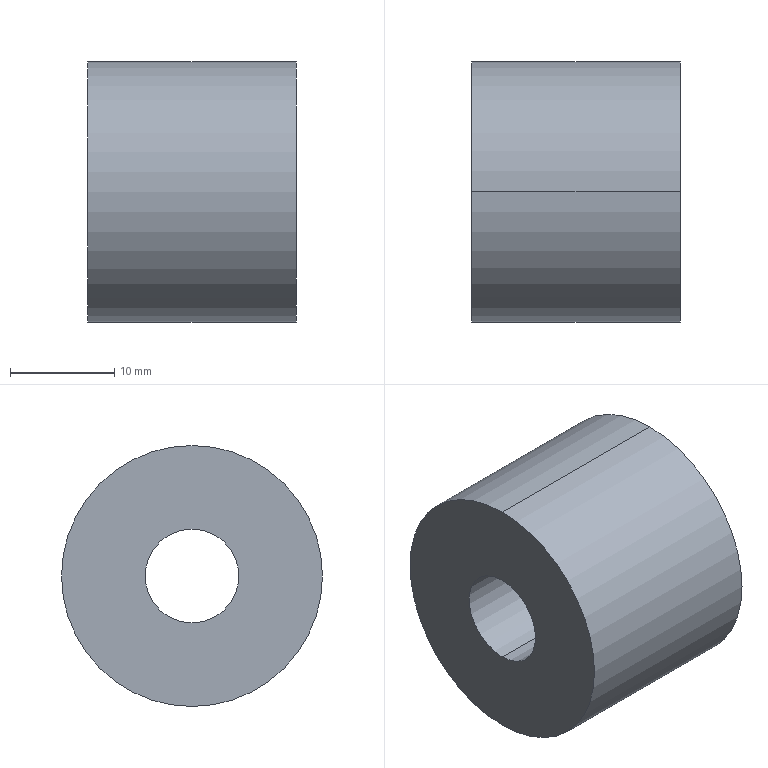Part | SolidWorks | features Extrusion 1, HoleWzd 1 | 1 solid | 9 faces | box 20 x 25 x 25 mm | volume 7188 mm3 | cylinder 6 | plane 3 | commonest cylinder face diameters 9 x2 15 x2 25 x2
STEP:
#1=CARTESIAN_POINT('',(8.,0.,7.5));
#2=VERTEX_POINT('',#1);
#3=CARTESIAN_POINT('',(8.,0.,-7.5));
#4=VERTEX_POINT('',#3);
#5=CARTESIAN_POINT('',(8.,0.,0.));
#6=DIRECTION('',(1.,0.,0.));
#7=DIRECTION('',(0.,0.,-1.));
#8=AXIS2_PLACEMENT_3D('',#5,#6,#7);
#9=CIRCLE('',#8,7.5);
#10=EDGE_CURVE('',#2,#4,#9,.T.);
#11=ORIENTED_EDGE('',*,*,#10,.F.);
#12=CARTESIAN_POINT('',(20.,0.,7.5));
#13=VERTEX_POINT('',#12);
#14=CARTESIAN_POINT('',(20.,0.,7.5));
#15=DIRECTION('',(1.,0.,0.));
#16=VECTOR('',#15,1000.);
#17=LINE('',#14,#16);
#18=EDGE_CURVE('',#2,#13,#17,.T.);
#19=ORIENTED_EDGE('',*,*,#18,.T.);
#20=CARTESIAN_POINT('',(20.,0.,-7.5));
#21=VERTEX_POINT('',#20);
#22=CARTESIAN_POINT('',(20.,0.,0.));
#23=DIRECTION('',(1.,0.,0.));
#24=DIRECTION('',(0.,0.,-1.));
#25=AXIS2_PLACEMENT_3D('',#22,#23,#24);
#26=CIRCLE('',#25,7.5);
#27=EDGE_CURVE('',#13,#21,#26,.T.);
#28=ORIENTED_EDGE('',*,*,#27,.T.);
#29=CARTESIAN_POINT('',(20.,0.,-7.5));
#30=DIRECTION('',(1.,0.,0.));
#31=VECTOR('',#30,1000.);
#32=LINE('',#29,#31);
#33=EDGE_CURVE('',#4,#21,#32,.T.);
#34=ORIENTED_EDGE('',*,*,#33,.F.);
#35=EDGE_LOOP('',(#11,#19,#28,#34));
#36=FACE_OUTER_BOUND('',#35,.T.);
#37=CARTESIAN_POINT('',(20.,0.,0.));
#38=DIRECTION('',(1.,0.,0.));
#39=DIRECTION('',(0.,0.,-1.));
#40=AXIS2_PLACEMENT_3D('',#37,#38,#39);
#41=CYLINDRICAL_SURFACE('',#40,7.5);
#42=ADVANCED_FACE('',(#36),#41,.F.);
#43=CARTESIAN_POINT('',(0.,0.,4.5));
#44=VERTEX_POINT('',#43);
#45=CARTESIAN_POINT('',(0.,0.,-4.5));
#46=VERTEX_POINT('',#45);
#47=CARTESIAN_POINT('',(0.,0.,0.));
#48=DIRECTION('',(1.,0.,0.));
#49=DIRECTION('',(0.,0.,-1.));
#50=AXIS2_PLACEMENT_3D('',#47,#48,#49);
#51=CIRCLE('',#50,4.5);
#52=EDGE_CURVE('',#44,#46,#51,.T.);
#53=ORIENTED_EDGE('',*,*,#52,.F.);
#54=CARTESIAN_POINT('',(8.,0.,4.5));
#55=VERTEX_POINT('',#54);
#56=CARTESIAN_POINT('',(20.,0.,4.5));
#57=DIRECTION('',(1.,0.,0.));
#58=VECTOR('',#57,1000.);
#59=LINE('',#56,#58);
#60=EDGE_CURVE('',#44,#55,#59,.T.);
#61=ORIENTED_EDGE('',*,*,#60,.T.);
#62=CARTESIAN_POINT('',(8.,0.,-4.5));
#63=VERTEX_POINT('',#62);
#64=CARTESIAN_POINT('',(8.,0.,0.));
#65=DIRECTION('',(1.,0.,0.));
#66=DIRECTION('',(0.,0.,-1.));
#67=AXIS2_PLACEMENT_3D('',#64,#65,#66);
#68=CIRCLE('',#67,4.5);
#69=EDGE_CURVE('',#55,#63,#68,.T.);
#70=ORIENTED_EDGE('',*,*,#69,.T.);
#71=CARTESIAN_POINT('',(20.,0.,-4.5));
#72=DIRECTION('',(1.,0.,0.));
#73=VECTOR('',#72,1000.);
#74=LINE('',#71,#73);
#75=EDGE_CURVE('',#46,#63,#74,.T.);
#76=ORIENTED_EDGE('',*,*,#75,.F.);
#77=EDGE_LOOP('',(#53,#61,#70,#76));
#78=FACE_OUTER_BOUND('',#77,.T.);
#79=CARTESIAN_POINT('',(20.,0.,0.));
#80=DIRECTION('',(1.,0.,0.));
#81=DIRECTION('',(0.,0.,-1.));
#82=AXIS2_PLACEMENT_3D('',#79,#80,#81);
#83=CYLINDRICAL_SURFACE('',#82,4.5);
#84=ADVANCED_FACE('',(#78),#83,.F.);
#85=CARTESIAN_POINT('',(20.,0.,-12.5));
#86=VERTEX_POINT('',#85);
#87=CARTESIAN_POINT('',(20.,0.,12.5));
#88=VERTEX_POINT('',#87);
#89=CARTESIAN_POINT('',(20.,0.,0.));
#90=DIRECTION('',(1.,0.,0.));
#91=DIRECTION('',(0.,0.,-1.));
#92=AXIS2_PLACEMENT_3D('',#89,#90,#91);
#93=CIRCLE('',#92,12.5);
#94=EDGE_CURVE('',#86,#88,#93,.T.);
#95=ORIENTED_EDGE('',*,*,#94,.F.);
#96=CARTESIAN_POINT('',(0.,0.,-12.5));
#97=VERTEX_POINT('',#96);
#98=CARTESIAN_POINT('',(20.,0.,-12.5));
#99=DIRECTION('',(-1.,0.,0.));
#100=VECTOR('',#99,1000.);
#101=LINE('',#98,#100);
#102=EDGE_CURVE('',#86,#97,#101,.T.);
#103=ORIENTED_EDGE('',*,*,#102,.T.);
#104=CARTESIAN_POINT('',(0.,0.,12.5));
#105=VERTEX_POINT('',#104);
#106=CARTESIAN_POINT('',(0.,0.,0.));
#107=DIRECTION('',(1.,0.,0.));
#108=DIRECTION('',(0.,0.,-1.));
#109=AXIS2_PLACEMENT_3D('',#106,#107,#108);
#110=CIRCLE('',#109,12.5);
#111=EDGE_CURVE('',#97,#105,#110,.T.);
#112=ORIENTED_EDGE('',*,*,#111,.T.);
#113=CARTESIAN_POINT('',(20.,0.,12.5));
#114=DIRECTION('',(-1.,0.,0.));
#115=VECTOR('',#114,1000.);
#116=LINE('',#113,#115);
#117=EDGE_CURVE('',#88,#105,#116,.T.);
#118=ORIENTED_EDGE('',*,*,#117,.F.);
#119=EDGE_LOOP('',(#95,#103,#112,#118));
#120=FACE_OUTER_BOUND('',#119,.T.);
#121=CARTESIAN_POINT('',(20.,0.,0.));
#122=DIRECTION('',(-1.,0.,0.));
#123=DIRECTION('',(0.,0.,1.));
#124=AXIS2_PLACEMENT_3D('',#121,#122,#123);
#125=CYLINDRICAL_SURFACE('',#124,12.5);
#126=ADVANCED_FACE('',(#120),#125,.T.);
#127=ORIENTED_EDGE('',*,*,#102,.F.);
#128=CARTESIAN_POINT('',(20.,0.,0.));
#129=DIRECTION('',(1.,0.,0.));
#130=DIRECTION('',(0.,0.,-1.));
#131=AXIS2_PLACEMENT_3D('',#128,#129,#130);
#132=CIRCLE('',#131,12.5);
#133=EDGE_CURVE('',#88,#86,#132,.T.);
#134=ORIENTED_EDGE('',*,*,#133,.F.);
#135=ORIENTED_EDGE('',*,*,#117,.T.);
#136=CARTESIAN_POINT('',(0.,0.,0.));
#137=DIRECTION('',(1.,0.,0.));
#138=DIRECTION('',(0.,0.,-1.));
#139=AXIS2_PLACEMENT_3D('',#136,#137,#138);
#140=CIRCLE('',#139,12.5);
#141=EDGE_CURVE('',#105,#97,#140,.T.);
#142=ORIENTED_EDGE('',*,*,#141,.T.);
#143=EDGE_LOOP('',(#127,#134,#135,#142));
#144=FACE_OUTER_BOUND('',#143,.T.);
#145=CARTESIAN_POINT('',(20.,0.,0.));
#146=DIRECTION('',(-1.,0.,0.));
#147=DIRECTION('',(0.,0.,1.));
#148=AXIS2_PLACEMENT_3D('',#145,#146,#147);
#149=CYLINDRICAL_SURFACE('',#148,12.5);
#150=ADVANCED_FACE('',(#144),#149,.T.);
#151=CARTESIAN_POINT('',(20.,0.,0.));
#152=DIRECTION('',(1.,0.,0.));
#153=DIRECTION('',(0.,0.,-1.));
#154=AXIS2_PLACEMENT_3D('',#151,#152,#153);
#155=CIRCLE('',#154,7.5);
#156=EDGE_CURVE('',#21,#13,#155,.T.);
#157=ORIENTED_EDGE('',*,*,#156,.F.);
#158=ORIENTED_EDGE('',*,*,#27,.F.);
#159=EDGE_LOOP('',(#157,#158));
#160=FACE_BOUND('',#159,.T.);
#161=ORIENTED_EDGE('',*,*,#133,.T.);
#162=ORIENTED_EDGE('',*,*,#94,.T.);
#163=EDGE_LOOP('',(#161,#162));
#164=FACE_OUTER_BOUND('',#163,.T.);
#165=CARTESIAN_POINT('',(20.,0.,0.));
#166=DIRECTION('',(1.,0.,0.));
#167=DIRECTION('',(0.,0.,-1.));
#168=AXIS2_PLACEMENT_3D('',#165,#166,#167);
#169=PLANE('',#168);
#170=ADVANCED_FACE('',(#160,#164),#169,.T.);
#171=CARTESIAN_POINT('',(0.,0.,0.));
#172=DIRECTION('',(1.,0.,0.));
#173=DIRECTION('',(0.,0.,-1.));
#174=AXIS2_PLACEMENT_3D('',#171,#172,#173);
#175=CIRCLE('',#174,4.5);
#176=EDGE_CURVE('',#46,#44,#175,.T.);
#177=ORIENTED_EDGE('',*,*,#176,.T.);
#178=ORIENTED_EDGE('',*,*,#52,.T.);
#179=EDGE_LOOP('',(#177,#178));
#180=FACE_BOUND('',#179,.T.);
#181=ORIENTED_EDGE('',*,*,#141,.F.);
#182=ORIENTED_EDGE('',*,*,#111,.F.);
#183=EDGE_LOOP('',(#181,#182));
#184=FACE_OUTER_BOUND('',#183,.T.);
#185=CARTESIAN_POINT('',(0.,0.,0.));
#186=DIRECTION('',(1.,0.,0.));
#187=DIRECTION('',(0.,0.,-1.));
#188=AXIS2_PLACEMENT_3D('',#185,#186,#187);
#189=PLANE('',#188);
#190=ADVANCED_FACE('',(#180,#184),#189,.F.);
#191=ORIENTED_EDGE('',*,*,#60,.F.);
#192=ORIENTED_EDGE('',*,*,#176,.F.);
#193=ORIENTED_EDGE('',*,*,#75,.T.);
#194=CARTESIAN_POINT('',(8.,0.,0.));
#195=DIRECTION('',(1.,0.,0.));
#196=DIRECTION('',(0.,0.,-1.));
#197=AXIS2_PLACEMENT_3D('',#194,#195,#196);
#198=CIRCLE('',#197,4.5);
#199=EDGE_CURVE('',#63,#55,#198,.T.);
#200=ORIENTED_EDGE('',*,*,#199,.T.);
#201=EDGE_LOOP('',(#191,#192,#193,#200));
#202=FACE_OUTER_BOUND('',#201,.T.);
#203=CARTESIAN_POINT('',(20.,0.,0.));
#204=DIRECTION('',(1.,0.,0.));
#205=DIRECTION('',(0.,0.,-1.));
#206=AXIS2_PLACEMENT_3D('',#203,#204,#205);
#207=CYLINDRICAL_SURFACE('',#206,4.5);
#208=ADVANCED_FACE('',(#202),#207,.F.);
#209=ORIENTED_EDGE('',*,*,#199,.F.);
#210=ORIENTED_EDGE('',*,*,#69,.F.);
#211=EDGE_LOOP('',(#209,#210));
#212=FACE_BOUND('',#211,.T.);
#213=CARTESIAN_POINT('',(8.,0.,0.));
#214=DIRECTION('',(1.,0.,0.));
#215=DIRECTION('',(0.,0.,-1.));
#216=AXIS2_PLACEMENT_3D('',#213,#214,#215);
#217=CIRCLE('',#216,7.5);
#218=EDGE_CURVE('',#4,#2,#217,.T.);
#219=ORIENTED_EDGE('',*,*,#218,.T.);
#220=ORIENTED_EDGE('',*,*,#10,.T.);
#221=EDGE_LOOP('',(#219,#220));
#222=FACE_OUTER_BOUND('',#221,.T.);
#223=CARTESIAN_POINT('',(8.,4.5,0.));
#224=DIRECTION('',(-1.,0.,0.));
#225=DIRECTION('',(0.,0.,1.));
#226=AXIS2_PLACEMENT_3D('',#223,#224,#225);
#227=PLANE('',#226);
#228=ADVANCED_FACE('',(#212,#222),#227,.F.);
#229=ORIENTED_EDGE('',*,*,#18,.F.);
#230=ORIENTED_EDGE('',*,*,#218,.F.);
#231=ORIENTED_EDGE('',*,*,#33,.T.);
#232=ORIENTED_EDGE('',*,*,#156,.T.);
#233=EDGE_LOOP('',(#229,#230,#231,#232));
#234=FACE_OUTER_BOUND('',#233,.T.);
#235=CARTESIAN_POINT('',(20.,0.,0.));
#236=DIRECTION('',(1.,0.,0.));
#237=DIRECTION('',(0.,0.,-1.));
#238=AXIS2_PLACEMENT_3D('',#235,#236,#237);
#239=CYLINDRICAL_SURFACE('',#238,7.5);
#240=ADVANCED_FACE('',(#234),#239,.F.);
#241=CLOSED_SHELL('',(#42,#84,#126,#150,#170,#190,#208,#228,#240));
#242=MANIFOLD_SOLID_BREP('',#241);
#243=CARTESIAN_POINT('',(0.,0.,0.));
#244=DIRECTION('',(0.,0.,1.));
#245=DIRECTION('',(1.,0.,0.));
#246=AXIS2_PLACEMENT_3D('',#243,#244,#245);
#247=(LENGTH_UNIT()NAMED_UNIT(*)SI_UNIT(.MILLI.,.METRE.));
#248=UNCERTAINTY_MEASURE_WITH_UNIT(LENGTH_MEASURE(0.00001),#247,'','');
#249=(NAMED_UNIT(*)PLANE_ANGLE_UNIT()SI_UNIT($,.RADIAN.));
#250=(NAMED_UNIT(*)SI_UNIT($,.STERADIAN.)SOLID_ANGLE_UNIT());
#251=(GEOMETRIC_REPRESENTATION_CONTEXT(3)GLOBAL_UNCERTAINTY_ASSIGNED_CONTEXT((#248))GLOBAL_UNIT_ASSIGNED_CONTEXT((#247,#249,#250))REPRESENTATION_CONTEXT('',''));
#252=ADVANCED_BREP_SHAPE_REPRESENTATION('',(#242,#246),#251);